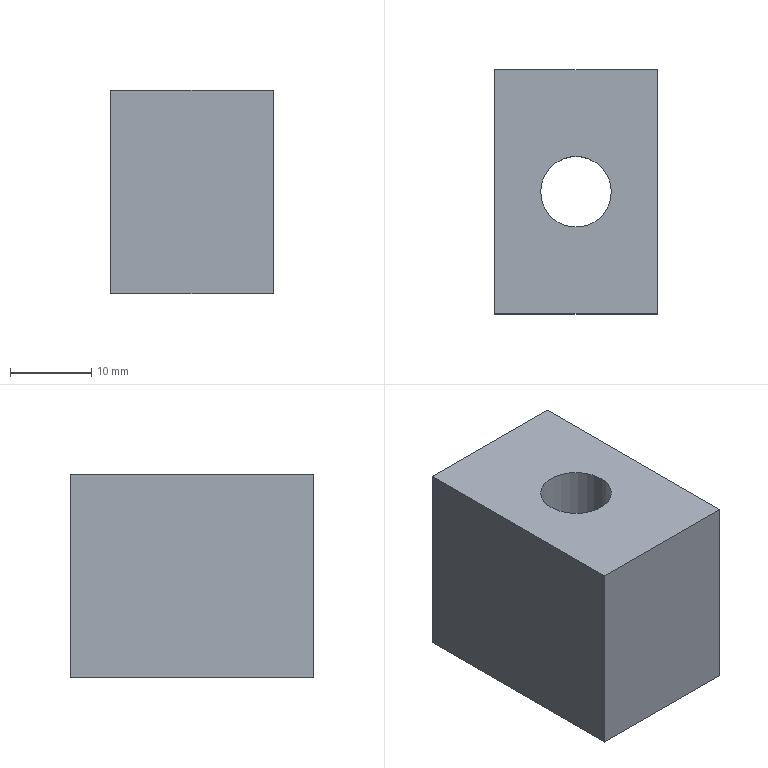Part | STEP file | 1_id1334_x_t | 1 solid | 11 faces | box 20 x 30 x 25 mm | volume 11989 mm3 | plane 7 | cylinder 4 | commonest cylinder face diameters 8.7 x2 15 x2
STEP:
#1=CARTESIAN_POINT('',(0.,0.,0.));
#2=DIRECTION('',(0.,0.,1.));
#3=DIRECTION('',(1.,0.,0.));
#4=AXIS2_PLACEMENT_3D('',#1,#2,#3);
#5=CARTESIAN_POINT('',(968.592,91.002,-86.54));
#6=VERTEX_POINT('',#5);
#7=CARTESIAN_POINT('',(948.592,91.002,-86.54));
#8=VERTEX_POINT('',#7);
#9=CARTESIAN_POINT('',(968.592,91.002,-86.54));
#10=DIRECTION('',(-1.,0.,0.));
#11=VECTOR('',#10,1.);
#12=LINE('',#9,#11);
#13=CARTESIAN_POINT('',(971.092,61.002,-86.54));
#14=DIRECTION('',(0.,0.,-1.));
#15=DIRECTION('',(1.,0.,0.));
#16=AXIS2_PLACEMENT_3D('',#13,#14,#15);
#17=PLANE('',#16);
#18=CARTESIAN_POINT('',(-2.5,-30.));
#19=DIRECTION('',(-1.,0.));
#20=VECTOR('',#19,1.);
#21=LINE('',#18,#20);
#22=(GEOMETRIC_REPRESENTATION_CONTEXT(2)PARAMETRIC_REPRESENTATION_CONTEXT()REPRESENTATION_CONTEXT('',''));
#23=DEFINITIONAL_REPRESENTATION('',(#21),#22);
#24=PCURVE('',#17,#23);
#25=CARTESIAN_POINT('',(946.092,91.002,-111.54));
#26=DIRECTION('',(0.,-1.,0.));
#27=DIRECTION('',(1.,0.,0.));
#28=AXIS2_PLACEMENT_3D('',#25,#26,#27);
#29=PLANE('',#28);
#30=CARTESIAN_POINT('',(22.5,25.));
#31=DIRECTION('',(-1.,0.));
#32=VECTOR('',#31,1.);
#33=LINE('',#30,#32);
#34=(GEOMETRIC_REPRESENTATION_CONTEXT(2)PARAMETRIC_REPRESENTATION_CONTEXT()REPRESENTATION_CONTEXT('',''));
#35=DEFINITIONAL_REPRESENTATION('',(#33),#34);
#36=PCURVE('',#29,#35);
#37=SURFACE_CURVE('',#12,(#24,#36),.PCURVE_S1.);
#38=EDGE_CURVE('',#6,#8,#37,.T.);
#39=ORIENTED_EDGE('',*,*,#38,.T.);
#40=CARTESIAN_POINT('',(948.592,61.002,-86.54));
#41=VERTEX_POINT('',#40);
#42=CARTESIAN_POINT('',(948.592,91.002,-86.54));
#43=DIRECTION('',(0.,-1.,0.));
#44=VECTOR('',#43,1.);
#45=LINE('',#42,#44);
#46=CARTESIAN_POINT('',(-22.5,-30.));
#47=DIRECTION('',(0.,1.));
#48=VECTOR('',#47,1.);
#49=LINE('',#46,#48);
#50=(GEOMETRIC_REPRESENTATION_CONTEXT(2)PARAMETRIC_REPRESENTATION_CONTEXT()REPRESENTATION_CONTEXT('',''));
#51=DEFINITIONAL_REPRESENTATION('',(#49),#50);
#52=PCURVE('',#17,#51);
#53=CARTESIAN_POINT('',(948.592,61.002,-111.54));
#54=DIRECTION('',(1.,0.,0.));
#55=DIRECTION('',(0.,0.,1.));
#56=AXIS2_PLACEMENT_3D('',#53,#54,#55);
#57=PLANE('',#56);
#58=CARTESIAN_POINT('',(25.,-30.));
#59=DIRECTION('',(0.,1.));
#60=VECTOR('',#59,1.);
#61=LINE('',#58,#60);
#62=(GEOMETRIC_REPRESENTATION_CONTEXT(2)PARAMETRIC_REPRESENTATION_CONTEXT()REPRESENTATION_CONTEXT('',''));
#63=DEFINITIONAL_REPRESENTATION('',(#61),#62);
#64=PCURVE('',#57,#63);
#65=SURFACE_CURVE('',#45,(#52,#64),.PCURVE_S1.);
#66=EDGE_CURVE('',#8,#41,#65,.T.);
#67=ORIENTED_EDGE('',*,*,#66,.T.);
#68=CARTESIAN_POINT('',(968.592,61.002,-86.54));
#69=VERTEX_POINT('',#68);
#70=CARTESIAN_POINT('',(948.592,61.002,-86.54));
#71=DIRECTION('',(1.,0.,0.));
#72=VECTOR('',#71,1.);
#73=LINE('',#70,#72);
#74=CARTESIAN_POINT('',(-22.5,0.));
#75=DIRECTION('',(1.,0.));
#76=VECTOR('',#75,1.);
#77=LINE('',#74,#76);
#78=(GEOMETRIC_REPRESENTATION_CONTEXT(2)PARAMETRIC_REPRESENTATION_CONTEXT()REPRESENTATION_CONTEXT('',''));
#79=DEFINITIONAL_REPRESENTATION('',(#77),#78);
#80=PCURVE('',#17,#79);
#81=CARTESIAN_POINT('',(971.092,61.002,-111.54));
#82=DIRECTION('',(0.,1.,0.));
#83=DIRECTION('',(0.,0.,-1.));
#84=AXIS2_PLACEMENT_3D('',#81,#82,#83);
#85=PLANE('',#84);
#86=CARTESIAN_POINT('',(-25.,22.5));
#87=DIRECTION('',(0.,-1.));
#88=VECTOR('',#87,1.);
#89=LINE('',#86,#88);
#90=(GEOMETRIC_REPRESENTATION_CONTEXT(2)PARAMETRIC_REPRESENTATION_CONTEXT()REPRESENTATION_CONTEXT('',''));
#91=DEFINITIONAL_REPRESENTATION('',(#89),#90);
#92=PCURVE('',#85,#91);
#93=SURFACE_CURVE('',#73,(#80,#92),.PCURVE_S1.);
#94=EDGE_CURVE('',#41,#69,#93,.T.);
#95=ORIENTED_EDGE('',*,*,#94,.T.);
#96=CARTESIAN_POINT('',(968.592,61.002,-86.54));
#97=DIRECTION('',(0.,1.,0.));
#98=VECTOR('',#97,1.);
#99=LINE('',#96,#98);
#100=CARTESIAN_POINT('',(-2.5,0.));
#101=DIRECTION('',(0.,-1.));
#102=VECTOR('',#101,1.);
#103=LINE('',#100,#102);
#104=(GEOMETRIC_REPRESENTATION_CONTEXT(2)PARAMETRIC_REPRESENTATION_CONTEXT()REPRESENTATION_CONTEXT('',''));
#105=DEFINITIONAL_REPRESENTATION('',(#103),#104);
#106=PCURVE('',#17,#105);
#107=CARTESIAN_POINT('',(968.592,91.002,-111.54));
#108=DIRECTION('',(-1.,0.,0.));
#109=DIRECTION('',(0.,1.,0.));
#110=AXIS2_PLACEMENT_3D('',#107,#108,#109);
#111=PLANE('',#110);
#112=CARTESIAN_POINT('',(-30.,-25.));
#113=DIRECTION('',(1.,0.));
#114=VECTOR('',#113,1.);
#115=LINE('',#112,#114);
#116=(GEOMETRIC_REPRESENTATION_CONTEXT(2)PARAMETRIC_REPRESENTATION_CONTEXT()REPRESENTATION_CONTEXT('',''));
#117=DEFINITIONAL_REPRESENTATION('',(#115),#116);
#118=PCURVE('',#111,#117);
#119=SURFACE_CURVE('',#99,(#106,#118),.PCURVE_S1.);
#120=EDGE_CURVE('',#69,#6,#119,.T.);
#121=ORIENTED_EDGE('',*,*,#120,.T.);
#122=EDGE_LOOP('',(#39,#67,#95,#121));
#123=FACE_BOUND('',#122,.T.);
#124=CARTESIAN_POINT('',(962.942,76.002,-86.54));
#125=VERTEX_POINT('',#124);
#126=CARTESIAN_POINT('',(954.242,76.002,-86.54));
#127=VERTEX_POINT('',#126);
#128=CARTESIAN_POINT('',(958.592,76.002,-86.54));
#129=DIRECTION('',(0.,0.,-1.));
#130=DIRECTION('',(1.,0.,0.));
#131=AXIS2_PLACEMENT_3D('',#128,#129,#130);
#132=CIRCLE('',#131,4.35);
#133=CARTESIAN_POINT('',(-12.5,-15.));
#134=DIRECTION('',(1.,0.));
#135=AXIS2_PLACEMENT_2D('',#133,#134);
#136=CIRCLE('',#135,4.35);
#137=(GEOMETRIC_REPRESENTATION_CONTEXT(2)PARAMETRIC_REPRESENTATION_CONTEXT()REPRESENTATION_CONTEXT('',''));
#138=DEFINITIONAL_REPRESENTATION('',(#136),#137);
#139=PCURVE('',#17,#138);
#140=CARTESIAN_POINT('',(958.592,76.002,-86.29));
#141=DIRECTION('',(0.,0.,1.));
#142=DIRECTION('',(1.,0.,0.));
#143=AXIS2_PLACEMENT_3D('',#140,#141,#142);
#144=CYLINDRICAL_SURFACE('',#143,4.35);
#145=CARTESIAN_POINT('',(6.283,-0.25));
#146=DIRECTION('',(-1.,0.));
#147=VECTOR('',#146,1.);
#148=LINE('',#145,#147);
#149=(GEOMETRIC_REPRESENTATION_CONTEXT(2)PARAMETRIC_REPRESENTATION_CONTEXT()REPRESENTATION_CONTEXT('',''));
#150=DEFINITIONAL_REPRESENTATION('',(#148),#149);
#151=PCURVE('',#144,#150);
#152=SURFACE_CURVE('',#132,(#139,#151),.PCURVE_S1.);
#153=EDGE_CURVE('',#125,#127,#152,.T.);
#154=ORIENTED_EDGE('',*,*,#153,.T.);
#155=CARTESIAN_POINT('',(958.592,76.002,-86.54));
#156=DIRECTION('',(0.,0.,-1.));
#157=DIRECTION('',(-1.,0.,0.));
#158=AXIS2_PLACEMENT_3D('',#155,#156,#157);
#159=CIRCLE('',#158,4.35);
#160=CARTESIAN_POINT('',(-12.5,-15.));
#161=DIRECTION('',(-1.,0.));
#162=AXIS2_PLACEMENT_2D('',#160,#161);
#163=CIRCLE('',#162,4.35);
#164=(GEOMETRIC_REPRESENTATION_CONTEXT(2)PARAMETRIC_REPRESENTATION_CONTEXT()REPRESENTATION_CONTEXT('',''));
#165=DEFINITIONAL_REPRESENTATION('',(#163),#164);
#166=PCURVE('',#17,#165);
#167=CARTESIAN_POINT('',(958.592,76.002,-86.29));
#168=DIRECTION('',(0.,0.,1.));
#169=DIRECTION('',(1.,0.,0.));
#170=AXIS2_PLACEMENT_3D('',#167,#168,#169);
#171=CYLINDRICAL_SURFACE('',#170,4.35);
#172=CARTESIAN_POINT('',(3.142,-0.25));
#173=DIRECTION('',(-1.,0.));
#174=VECTOR('',#173,1.);
#175=LINE('',#172,#174);
#176=(GEOMETRIC_REPRESENTATION_CONTEXT(2)PARAMETRIC_REPRESENTATION_CONTEXT()REPRESENTATION_CONTEXT('',''));
#177=DEFINITIONAL_REPRESENTATION('',(#175),#176);
#178=PCURVE('',#171,#177);
#179=SURFACE_CURVE('',#159,(#166,#178),.PCURVE_S1.);
#180=EDGE_CURVE('',#127,#125,#179,.T.);
#181=ORIENTED_EDGE('',*,*,#180,.T.);
#182=EDGE_LOOP('',(#154,#181));
#183=FACE_BOUND('',#182,.T.);
#184=ADVANCED_FACE('',(#123,#183),#17,.F.);
#185=CARTESIAN_POINT('',(968.592,61.002,-111.54));
#186=VERTEX_POINT('',#185);
#187=CARTESIAN_POINT('',(968.592,61.002,-86.54));
#188=DIRECTION('',(0.,0.,-1.));
#189=VECTOR('',#188,1.);
#190=LINE('',#187,#189);
#191=CARTESIAN_POINT('',(-30.,-25.));
#192=DIRECTION('',(0.,1.));
#193=VECTOR('',#192,1.);
#194=LINE('',#191,#193);
#195=(GEOMETRIC_REPRESENTATION_CONTEXT(2)PARAMETRIC_REPRESENTATION_CONTEXT()REPRESENTATION_CONTEXT('',''));
#196=DEFINITIONAL_REPRESENTATION('',(#194),#195);
#197=PCURVE('',#111,#196);
#198=CARTESIAN_POINT('',(-25.,2.5));
#199=DIRECTION('',(1.,0.));
#200=VECTOR('',#199,1.);
#201=LINE('',#198,#200);
#202=(GEOMETRIC_REPRESENTATION_CONTEXT(2)PARAMETRIC_REPRESENTATION_CONTEXT()REPRESENTATION_CONTEXT('',''));
#203=DEFINITIONAL_REPRESENTATION('',(#201),#202);
#204=PCURVE('',#85,#203);
#205=SURFACE_CURVE('',#190,(#197,#204),.PCURVE_S1.);
#206=EDGE_CURVE('',#69,#186,#205,.T.);
#207=ORIENTED_EDGE('',*,*,#206,.T.);
#208=CARTESIAN_POINT('',(968.592,91.002,-111.54));
#209=VERTEX_POINT('',#208);
#210=CARTESIAN_POINT('',(968.592,61.002,-111.54));
#211=DIRECTION('',(0.,1.,0.));
#212=VECTOR('',#211,1.);
#213=LINE('',#210,#212);
#214=CARTESIAN_POINT('',(-30.,0.));
#215=DIRECTION('',(1.,0.));
#216=VECTOR('',#215,1.);
#217=LINE('',#214,#216);
#218=(GEOMETRIC_REPRESENTATION_CONTEXT(2)PARAMETRIC_REPRESENTATION_CONTEXT()REPRESENTATION_CONTEXT('',''));
#219=DEFINITIONAL_REPRESENTATION('',(#217),#218);
#220=PCURVE('',#111,#219);
#221=CARTESIAN_POINT('',(971.092,61.002,-111.54));
#222=DIRECTION('',(0.,0.,-1.));
#223=DIRECTION('',(1.,0.,0.));
#224=AXIS2_PLACEMENT_3D('',#221,#222,#223);
#225=PLANE('',#224);
#226=CARTESIAN_POINT('',(-2.5,0.));
#227=DIRECTION('',(0.,-1.));
#228=VECTOR('',#227,1.);
#229=LINE('',#226,#228);
#230=(GEOMETRIC_REPRESENTATION_CONTEXT(2)PARAMETRIC_REPRESENTATION_CONTEXT()REPRESENTATION_CONTEXT('',''));
#231=DEFINITIONAL_REPRESENTATION('',(#229),#230);
#232=PCURVE('',#225,#231);
#233=SURFACE_CURVE('',#213,(#220,#232),.PCURVE_S1.);
#234=EDGE_CURVE('',#186,#209,#233,.T.);
#235=ORIENTED_EDGE('',*,*,#234,.T.);
#236=CARTESIAN_POINT('',(968.592,91.002,-86.54));
#237=DIRECTION('',(0.,0.,-1.));
#238=VECTOR('',#237,1.);
#239=LINE('',#236,#238);
#240=CARTESIAN_POINT('',(0.,-25.));
#241=DIRECTION('',(0.,1.));
#242=VECTOR('',#241,1.);
#243=LINE('',#240,#242);
#244=(GEOMETRIC_REPRESENTATION_CONTEXT(2)PARAMETRIC_REPRESENTATION_CONTEXT()REPRESENTATION_CONTEXT('',''));
#245=DEFINITIONAL_REPRESENTATION('',(#243),#244);
#246=PCURVE('',#111,#245);
#247=CARTESIAN_POINT('',(22.5,25.));
#248=DIRECTION('',(0.,-1.));
#249=VECTOR('',#248,1.);
#250=LINE('',#247,#249);
#251=(GEOMETRIC_REPRESENTATION_CONTEXT(2)PARAMETRIC_REPRESENTATION_CONTEXT()REPRESENTATION_CONTEXT('',''));
#252=DEFINITIONAL_REPRESENTATION('',(#250),#251);
#253=PCURVE('',#29,#252);
#254=SURFACE_CURVE('',#239,(#246,#253),.PCURVE_S1.);
#255=EDGE_CURVE('',#6,#209,#254,.T.);
#256=ORIENTED_EDGE('',*,*,#255,.F.);
#257=ORIENTED_EDGE('',*,*,#120,.F.);
#258=EDGE_LOOP('',(#207,#235,#256,#257));
#259=FACE_BOUND('',#258,.T.);
#260=ADVANCED_FACE('',(#259),#111,.F.);
#261=ORIENTED_EDGE('',*,*,#255,.T.);
#262=CARTESIAN_POINT('',(948.592,91.002,-111.54));
#263=VERTEX_POINT('',#262);
#264=CARTESIAN_POINT('',(968.592,91.002,-111.54));
#265=DIRECTION('',(-1.,0.,0.));
#266=VECTOR('',#265,1.);
#267=LINE('',#264,#266);
#268=CARTESIAN_POINT('',(22.5,0.));
#269=DIRECTION('',(-1.,0.));
#270=VECTOR('',#269,1.);
#271=LINE('',#268,#270);
#272=(GEOMETRIC_REPRESENTATION_CONTEXT(2)PARAMETRIC_REPRESENTATION_CONTEXT()REPRESENTATION_CONTEXT('',''));
#273=DEFINITIONAL_REPRESENTATION('',(#271),#272);
#274=PCURVE('',#29,#273);
#275=CARTESIAN_POINT('',(-2.5,-30.));
#276=DIRECTION('',(-1.,0.));
#277=VECTOR('',#276,1.);
#278=LINE('',#275,#277);
#279=(GEOMETRIC_REPRESENTATION_CONTEXT(2)PARAMETRIC_REPRESENTATION_CONTEXT()REPRESENTATION_CONTEXT('',''));
#280=DEFINITIONAL_REPRESENTATION('',(#278),#279);
#281=PCURVE('',#225,#280);
#282=SURFACE_CURVE('',#267,(#274,#281),.PCURVE_S1.);
#283=EDGE_CURVE('',#209,#263,#282,.T.);
#284=ORIENTED_EDGE('',*,*,#283,.T.);
#285=CARTESIAN_POINT('',(948.592,91.002,-86.54));
#286=DIRECTION('',(0.,0.,-1.));
#287=VECTOR('',#286,1.);
#288=LINE('',#285,#287);
#289=CARTESIAN_POINT('',(2.5,25.));
#290=DIRECTION('',(0.,-1.));
#291=VECTOR('',#290,1.);
#292=LINE('',#289,#291);
#293=(GEOMETRIC_REPRESENTATION_CONTEXT(2)PARAMETRIC_REPRESENTATION_CONTEXT()REPRESENTATION_CONTEXT('',''));
#294=DEFINITIONAL_REPRESENTATION('',(#292),#293);
#295=PCURVE('',#29,#294);
#296=CARTESIAN_POINT('',(25.,-30.));
#297=DIRECTION('',(-1.,0.));
#298=VECTOR('',#297,1.);
#299=LINE('',#296,#298);
#300=(GEOMETRIC_REPRESENTATION_CONTEXT(2)PARAMETRIC_REPRESENTATION_CONTEXT()REPRESENTATION_CONTEXT('',''));
#301=DEFINITIONAL_REPRESENTATION('',(#299),#300);
#302=PCURVE('',#57,#301);
#303=SURFACE_CURVE('',#288,(#295,#302),.PCURVE_S1.);
#304=EDGE_CURVE('',#8,#263,#303,.T.);
#305=ORIENTED_EDGE('',*,*,#304,.F.);
#306=ORIENTED_EDGE('',*,*,#38,.F.);
#307=EDGE_LOOP('',(#261,#284,#305,#306));
#308=FACE_BOUND('',#307,.T.);
#309=ADVANCED_FACE('',(#308),#29,.F.);
#310=ORIENTED_EDGE('',*,*,#304,.T.);
#311=CARTESIAN_POINT('',(948.592,61.002,-111.54));
#312=VERTEX_POINT('',#311);
#313=CARTESIAN_POINT('',(948.592,91.002,-111.54));
#314=DIRECTION('',(0.,-1.,0.));
#315=VECTOR('',#314,1.);
#316=LINE('',#313,#315);
#317=CARTESIAN_POINT('',(0.,-30.));
#318=DIRECTION('',(0.,1.));
#319=VECTOR('',#318,1.);
#320=LINE('',#317,#319);
#321=(GEOMETRIC_REPRESENTATION_CONTEXT(2)PARAMETRIC_REPRESENTATION_CONTEXT()REPRESENTATION_CONTEXT('',''));
#322=DEFINITIONAL_REPRESENTATION('',(#320),#321);
#323=PCURVE('',#57,#322);
#324=CARTESIAN_POINT('',(-22.5,-30.));
#325=DIRECTION('',(0.,1.));
#326=VECTOR('',#325,1.);
#327=LINE('',#324,#326);
#328=(GEOMETRIC_REPRESENTATION_CONTEXT(2)PARAMETRIC_REPRESENTATION_CONTEXT()REPRESENTATION_CONTEXT('',''));
#329=DEFINITIONAL_REPRESENTATION('',(#327),#328);
#330=PCURVE('',#225,#329);
#331=SURFACE_CURVE('',#316,(#323,#330),.PCURVE_S1.);
#332=EDGE_CURVE('',#263,#312,#331,.T.);
#333=ORIENTED_EDGE('',*,*,#332,.T.);
#334=CARTESIAN_POINT('',(948.592,61.002,-86.54));
#335=DIRECTION('',(0.,0.,-1.));
#336=VECTOR('',#335,1.);
#337=LINE('',#334,#336);
#338=CARTESIAN_POINT('',(25.,0.));
#339=DIRECTION('',(-1.,0.));
#340=VECTOR('',#339,1.);
#341=LINE('',#338,#340);
#342=(GEOMETRIC_REPRESENTATION_CONTEXT(2)PARAMETRIC_REPRESENTATION_CONTEXT()REPRESENTATION_CONTEXT('',''));
#343=DEFINITIONAL_REPRESENTATION('',(#341),#342);
#344=PCURVE('',#57,#343);
#345=CARTESIAN_POINT('',(-25.,22.5));
#346=DIRECTION('',(1.,0.));
#347=VECTOR('',#346,1.);
#348=LINE('',#345,#347);
#349=(GEOMETRIC_REPRESENTATION_CONTEXT(2)PARAMETRIC_REPRESENTATION_CONTEXT()REPRESENTATION_CONTEXT('',''));
#350=DEFINITIONAL_REPRESENTATION('',(#348),#349);
#351=PCURVE('',#85,#350);
#352=SURFACE_CURVE('',#337,(#344,#351),.PCURVE_S1.);
#353=EDGE_CURVE('',#41,#312,#352,.T.);
#354=ORIENTED_EDGE('',*,*,#353,.F.);
#355=ORIENTED_EDGE('',*,*,#66,.F.);
#356=EDGE_LOOP('',(#310,#333,#354,#355));
#357=FACE_BOUND('',#356,.T.);
#358=ADVANCED_FACE('',(#357),#57,.F.);
#359=ORIENTED_EDGE('',*,*,#353,.T.);
#360=CARTESIAN_POINT('',(948.592,61.002,-111.54));
#361=DIRECTION('',(1.,0.,0.));
#362=VECTOR('',#361,1.);
#363=LINE('',#360,#362);
#364=CARTESIAN_POINT('',(0.,22.5));
#365=DIRECTION('',(0.,-1.));
#366=VECTOR('',#365,1.);
#367=LINE('',#364,#366);
#368=(GEOMETRIC_REPRESENTATION_CONTEXT(2)PARAMETRIC_REPRESENTATION_CONTEXT()REPRESENTATION_CONTEXT('',''));
#369=DEFINITIONAL_REPRESENTATION('',(#367),#368);
#370=PCURVE('',#85,#369);
#371=CARTESIAN_POINT('',(-22.5,0.));
#372=DIRECTION('',(1.,0.));
#373=VECTOR('',#372,1.);
#374=LINE('',#371,#373);
#375=(GEOMETRIC_REPRESENTATION_CONTEXT(2)PARAMETRIC_REPRESENTATION_CONTEXT()REPRESENTATION_CONTEXT('',''));
#376=DEFINITIONAL_REPRESENTATION('',(#374),#375);
#377=PCURVE('',#225,#376);
#378=SURFACE_CURVE('',#363,(#370,#377),.PCURVE_S1.);
#379=EDGE_CURVE('',#312,#186,#378,.T.);
#380=ORIENTED_EDGE('',*,*,#379,.T.);
#381=ORIENTED_EDGE('',*,*,#206,.F.);
#382=ORIENTED_EDGE('',*,*,#94,.F.);
#383=EDGE_LOOP('',(#359,#380,#381,#382));
#384=FACE_BOUND('',#383,.T.);
#385=ADVANCED_FACE('',(#384),#85,.F.);
#386=ORIENTED_EDGE('',*,*,#379,.F.);
#387=ORIENTED_EDGE('',*,*,#332,.F.);
#388=ORIENTED_EDGE('',*,*,#283,.F.);
#389=ORIENTED_EDGE('',*,*,#234,.F.);
#390=EDGE_LOOP('',(#386,#387,#388,#389));
#391=FACE_BOUND('',#390,.T.);
#392=CARTESIAN_POINT('',(966.092,76.002,-111.54));
#393=VERTEX_POINT('',#392);
#394=CARTESIAN_POINT('',(951.092,76.002,-111.54));
#395=VERTEX_POINT('',#394);
#396=CARTESIAN_POINT('',(958.592,76.002,-111.54));
#397=DIRECTION('',(0.,0.,1.));
#398=DIRECTION('',(1.,0.,0.));
#399=AXIS2_PLACEMENT_3D('',#396,#397,#398);
#400=CIRCLE('',#399,7.5);
#401=CARTESIAN_POINT('',(-5.,-15.));
#402=CARTESIAN_POINT('',(-5.,-27.99));
#403=CARTESIAN_POINT('',(-16.25,-21.495));
#404=CARTESIAN_POINT('',(-27.5,-15.));
#405=CARTESIAN_POINT('',(-16.25,-8.505));
#406=CARTESIAN_POINT('',(-5.,-2.01));
#407=CARTESIAN_POINT('',(-5.,-15.));
#408=(BOUNDED_CURVE()B_SPLINE_CURVE(2,(#401,#402,#403,#404,#405,#406,#407),.UNSPECIFIED.,.T.,.F.)B_SPLINE_CURVE_WITH_KNOTS((1,2,2,2,2,1),(-2.094,0.,2.094,4.189,6.283,8.378),.UNSPECIFIED.)CURVE()GEOMETRIC_REPRESENTATION_ITEM()RATIONAL_B_SPLINE_CURVE((1.,0.5,1.,0.5,1.,0.5,1.))REPRESENTATION_ITEM(''));
#409=(GEOMETRIC_REPRESENTATION_CONTEXT(2)PARAMETRIC_REPRESENTATION_CONTEXT()REPRESENTATION_CONTEXT('',''));
#410=DEFINITIONAL_REPRESENTATION('',(#408),#409);
#411=PCURVE('',#225,#410);
#412=CARTESIAN_POINT('',(958.592,76.002,-98.54));
#413=DIRECTION('',(0.,0.,1.));
#414=DIRECTION('',(1.,0.,0.));
#415=AXIS2_PLACEMENT_3D('',#412,#413,#414);
#416=CYLINDRICAL_SURFACE('',#415,7.5);
#417=CARTESIAN_POINT('',(0.,-13.));
#418=DIRECTION('',(1.,0.));
#419=VECTOR('',#418,1.);
#420=LINE('',#417,#419);
#421=(GEOMETRIC_REPRESENTATION_CONTEXT(2)PARAMETRIC_REPRESENTATION_CONTEXT()REPRESENTATION_CONTEXT('',''));
#422=DEFINITIONAL_REPRESENTATION('',(#420),#421);
#423=PCURVE('',#416,#422);
#424=SURFACE_CURVE('',#400,(#411,#423),.PCURVE_S1.);
#425=EDGE_CURVE('',#393,#395,#424,.T.);
#426=ORIENTED_EDGE('',*,*,#425,.T.);
#427=CARTESIAN_POINT('',(958.592,76.002,-111.54));
#428=DIRECTION('',(0.,0.,1.));
#429=DIRECTION('',(-1.,0.,0.));
#430=AXIS2_PLACEMENT_3D('',#427,#428,#429);
#431=CIRCLE('',#430,7.5);
#432=CARTESIAN_POINT('',(-20.,-15.));
#433=CARTESIAN_POINT('',(-20.,-2.01));
#434=CARTESIAN_POINT('',(-8.75,-8.505));
#435=CARTESIAN_POINT('',(2.5,-15.));
#436=CARTESIAN_POINT('',(-8.75,-21.495));
#437=CARTESIAN_POINT('',(-20.,-27.99));
#438=CARTESIAN_POINT('',(-20.,-15.));
#439=(BOUNDED_CURVE()B_SPLINE_CURVE(2,(#432,#433,#434,#435,#436,#437,#438),.UNSPECIFIED.,.T.,.F.)B_SPLINE_CURVE_WITH_KNOTS((1,2,2,2,2,1),(-2.094,0.,2.094,4.189,6.283,8.378),.UNSPECIFIED.)CURVE()GEOMETRIC_REPRESENTATION_ITEM()RATIONAL_B_SPLINE_CURVE((1.,0.5,1.,0.5,1.,0.5,1.))REPRESENTATION_ITEM(''));
#440=(GEOMETRIC_REPRESENTATION_CONTEXT(2)PARAMETRIC_REPRESENTATION_CONTEXT()REPRESENTATION_CONTEXT('',''));
#441=DEFINITIONAL_REPRESENTATION('',(#439),#440);
#442=PCURVE('',#225,#441);
#443=CARTESIAN_POINT('',(958.592,76.002,-98.54));
#444=DIRECTION('',(0.,0.,1.));
#445=DIRECTION('',(1.,0.,0.));
#446=AXIS2_PLACEMENT_3D('',#443,#444,#445);
#447=CYLINDRICAL_SURFACE('',#446,7.5);
#448=CARTESIAN_POINT('',(3.142,-13.));
#449=DIRECTION('',(1.,0.));
#450=VECTOR('',#449,1.);
#451=LINE('',#448,#450);
#452=(GEOMETRIC_REPRESENTATION_CONTEXT(2)PARAMETRIC_REPRESENTATION_CONTEXT()REPRESENTATION_CONTEXT('',''));
#453=DEFINITIONAL_REPRESENTATION('',(#451),#452);
#454=PCURVE('',#447,#453);
#455=SURFACE_CURVE('',#431,(#442,#454),.PCURVE_S1.);
#456=EDGE_CURVE('',#395,#393,#455,.T.);
#457=ORIENTED_EDGE('',*,*,#456,.T.);
#458=EDGE_LOOP('',(#426,#457));
#459=FACE_BOUND('',#458,.T.);
#460=ADVANCED_FACE('',(#391,#459),#225,.T.);
#461=CARTESIAN_POINT('',(966.092,76.002,-98.54));
#462=VERTEX_POINT('',#461);
#463=CARTESIAN_POINT('',(951.092,76.002,-98.54));
#464=VERTEX_POINT('',#463);
#465=CARTESIAN_POINT('',(958.592,76.002,-98.54));
#466=DIRECTION('',(0.,0.,-1.));
#467=DIRECTION('',(1.,0.,0.));
#468=AXIS2_PLACEMENT_3D('',#465,#466,#467);
#469=CIRCLE('',#468,7.5);
#470=CARTESIAN_POINT('',(6.283,0.));
#471=DIRECTION('',(-1.,0.));
#472=VECTOR('',#471,1.);
#473=LINE('',#470,#472);
#474=(GEOMETRIC_REPRESENTATION_CONTEXT(2)PARAMETRIC_REPRESENTATION_CONTEXT()REPRESENTATION_CONTEXT('',''));
#475=DEFINITIONAL_REPRESENTATION('',(#473),#474);
#476=PCURVE('',#447,#475);
#477=CARTESIAN_POINT('',(958.592,76.002,-98.54));
#478=DIRECTION('',(0.,0.,1.));
#479=DIRECTION('',(0.,-1.,0.));
#480=AXIS2_PLACEMENT_3D('',#477,#478,#479);
#481=PLANE('',#480);
#482=CARTESIAN_POINT('',(0.,7.5));
#483=CARTESIAN_POINT('',(12.99,7.5));
#484=CARTESIAN_POINT('',(6.495,-3.75));
#485=CARTESIAN_POINT('',(0.,-15.));
#486=CARTESIAN_POINT('',(-6.495,-3.75));
#487=CARTESIAN_POINT('',(-12.99,7.5));
#488=CARTESIAN_POINT('',(0.,7.5));
#489=(BOUNDED_CURVE()B_SPLINE_CURVE(2,(#482,#483,#484,#485,#486,#487,#488),.UNSPECIFIED.,.T.,.F.)B_SPLINE_CURVE_WITH_KNOTS((1,2,2,2,2,1),(-2.094,0.,2.094,4.189,6.283,8.378),.UNSPECIFIED.)CURVE()GEOMETRIC_REPRESENTATION_ITEM()RATIONAL_B_SPLINE_CURVE((1.,0.5,1.,0.5,1.,0.5,1.))REPRESENTATION_ITEM(''));
#490=(GEOMETRIC_REPRESENTATION_CONTEXT(2)PARAMETRIC_REPRESENTATION_CONTEXT()REPRESENTATION_CONTEXT('',''));
#491=DEFINITIONAL_REPRESENTATION('',(#489),#490);
#492=PCURVE('',#481,#491);
#493=SURFACE_CURVE('',#469,(#476,#492),.PCURVE_S1.);
#494=EDGE_CURVE('',#462,#464,#493,.T.);
#495=ORIENTED_EDGE('',*,*,#494,.T.);
#496=CARTESIAN_POINT('',(951.092,76.002,-111.54));
#497=DIRECTION('',(0.,0.,-1.));
#498=VECTOR('',#497,1.);
#499=LINE('',#496,#498);
#500=CARTESIAN_POINT('',(3.142,-13.));
#501=DIRECTION('',(0.,-1.));
#502=VECTOR('',#501,1.);
#503=LINE('',#500,#502);
#504=(GEOMETRIC_REPRESENTATION_CONTEXT(2)PARAMETRIC_REPRESENTATION_CONTEXT()REPRESENTATION_CONTEXT('',''));
#505=DEFINITIONAL_REPRESENTATION('',(#503),#504);
#506=PCURVE('',#447,#505);
#507=CARTESIAN_POINT('',(3.142,-13.));
#508=DIRECTION('',(0.,-1.));
#509=VECTOR('',#508,1.);
#510=LINE('',#507,#509);
#511=(GEOMETRIC_REPRESENTATION_CONTEXT(2)PARAMETRIC_REPRESENTATION_CONTEXT()REPRESENTATION_CONTEXT('',''));
#512=DEFINITIONAL_REPRESENTATION('',(#510),#511);
#513=PCURVE('',#416,#512);
#514=SURFACE_CURVE('',#499,(#506,#513),.PCURVE_S1.);
#515=EDGE_CURVE('',#464,#395,#514,.T.);
#516=ORIENTED_EDGE('',*,*,#515,.T.);
#517=ORIENTED_EDGE('',*,*,#456,.T.);
#518=CARTESIAN_POINT('',(966.092,76.002,-111.54));
#519=DIRECTION('',(0.,0.,1.));
#520=VECTOR('',#519,1.);
#521=LINE('',#518,#520);
#522=CARTESIAN_POINT('',(6.283,-13.));
#523=DIRECTION('',(0.,1.));
#524=VECTOR('',#523,1.);
#525=LINE('',#522,#524);
#526=(GEOMETRIC_REPRESENTATION_CONTEXT(2)PARAMETRIC_REPRESENTATION_CONTEXT()REPRESENTATION_CONTEXT('',''));
#527=DEFINITIONAL_REPRESENTATION('',(#525),#526);
#528=PCURVE('',#447,#527);
#529=CARTESIAN_POINT('',(0.,-13.));
#530=DIRECTION('',(0.,1.));
#531=VECTOR('',#530,1.);
#532=LINE('',#529,#531);
#533=(GEOMETRIC_REPRESENTATION_CONTEXT(2)PARAMETRIC_REPRESENTATION_CONTEXT()REPRESENTATION_CONTEXT('',''));
#534=DEFINITIONAL_REPRESENTATION('',(#532),#533);
#535=PCURVE('',#416,#534);
#536=SURFACE_CURVE('',#521,(#528,#535),.PCURVE_S1.);
#537=EDGE_CURVE('',#393,#462,#536,.T.);
#538=ORIENTED_EDGE('',*,*,#537,.T.);
#539=EDGE_LOOP('',(#495,#516,#517,#538));
#540=FACE_BOUND('',#539,.F.);
#541=ADVANCED_FACE('',(#540),#447,.F.);
#542=ORIENTED_EDGE('',*,*,#494,.T.);
#543=CARTESIAN_POINT('',(958.592,76.002,-98.54));
#544=DIRECTION('',(0.,0.,-1.));
#545=DIRECTION('',(-1.,0.,0.));
#546=AXIS2_PLACEMENT_3D('',#543,#544,#545);
#547=CIRCLE('',#546,7.5);
#548=CARTESIAN_POINT('',(0.,-7.5));
#549=CARTESIAN_POINT('',(-12.99,-7.5));
#550=CARTESIAN_POINT('',(-6.495,3.75));
#551=CARTESIAN_POINT('',(0.,15.));
#552=CARTESIAN_POINT('',(6.495,3.75));
#553=CARTESIAN_POINT('',(12.99,-7.5));
#554=CARTESIAN_POINT('',(0.,-7.5));
#555=(BOUNDED_CURVE()B_SPLINE_CURVE(2,(#548,#549,#550,#551,#552,#553,#554),.UNSPECIFIED.,.T.,.F.)B_SPLINE_CURVE_WITH_KNOTS((1,2,2,2,2,1),(-2.094,0.,2.094,4.189,6.283,8.378),.UNSPECIFIED.)CURVE()GEOMETRIC_REPRESENTATION_ITEM()RATIONAL_B_SPLINE_CURVE((1.,0.5,1.,0.5,1.,0.5,1.))REPRESENTATION_ITEM(''));
#556=(GEOMETRIC_REPRESENTATION_CONTEXT(2)PARAMETRIC_REPRESENTATION_CONTEXT()REPRESENTATION_CONTEXT('',''));
#557=DEFINITIONAL_REPRESENTATION('',(#555),#556);
#558=PCURVE('',#481,#557);
#559=CARTESIAN_POINT('',(3.142,0.));
#560=DIRECTION('',(-1.,0.));
#561=VECTOR('',#560,1.);
#562=LINE('',#559,#561);
#563=(GEOMETRIC_REPRESENTATION_CONTEXT(2)PARAMETRIC_REPRESENTATION_CONTEXT()REPRESENTATION_CONTEXT('',''));
#564=DEFINITIONAL_REPRESENTATION('',(#562),#563);
#565=PCURVE('',#416,#564);
#566=SURFACE_CURVE('',#547,(#558,#565),.PCURVE_S1.);
#567=EDGE_CURVE('',#464,#462,#566,.T.);
#568=ORIENTED_EDGE('',*,*,#567,.T.);
#569=EDGE_LOOP('',(#542,#568));
#570=FACE_BOUND('',#569,.T.);
#571=CARTESIAN_POINT('',(954.242,76.002,-98.54));
#572=VERTEX_POINT('',#571);
#573=CARTESIAN_POINT('',(962.942,76.002,-98.54));
#574=VERTEX_POINT('',#573);
#575=CARTESIAN_POINT('',(958.592,76.002,-98.54));
#576=DIRECTION('',(0.,0.,1.));
#577=DIRECTION('',(-1.,0.,0.));
#578=AXIS2_PLACEMENT_3D('',#575,#576,#577);
#579=CIRCLE('',#578,4.35);
#580=CARTESIAN_POINT('',(0.,0.));
#581=DIRECTION('',(0.,-1.));
#582=AXIS2_PLACEMENT_2D('',#580,#581);
#583=CIRCLE('',#582,4.35);
#584=(GEOMETRIC_REPRESENTATION_CONTEXT(2)PARAMETRIC_REPRESENTATION_CONTEXT()REPRESENTATION_CONTEXT('',''));
#585=DEFINITIONAL_REPRESENTATION('',(#583),#584);
#586=PCURVE('',#481,#585);
#587=CARTESIAN_POINT('',(3.142,-12.25));
#588=DIRECTION('',(1.,0.));
#589=VECTOR('',#588,1.);
#590=LINE('',#587,#589);
#591=(GEOMETRIC_REPRESENTATION_CONTEXT(2)PARAMETRIC_REPRESENTATION_CONTEXT()REPRESENTATION_CONTEXT('',''));
#592=DEFINITIONAL_REPRESENTATION('',(#590),#591);
#593=PCURVE('',#144,#592);
#594=SURFACE_CURVE('',#579,(#586,#593),.PCURVE_S1.);
#595=EDGE_CURVE('',#572,#574,#594,.T.);
#596=ORIENTED_EDGE('',*,*,#595,.T.);
#597=CARTESIAN_POINT('',(958.592,76.002,-98.54));
#598=DIRECTION('',(0.,0.,1.));
#599=DIRECTION('',(1.,0.,0.));
#600=AXIS2_PLACEMENT_3D('',#597,#598,#599);
#601=CIRCLE('',#600,4.35);
#602=CARTESIAN_POINT('',(0.,0.));
#603=DIRECTION('',(0.,1.));
#604=AXIS2_PLACEMENT_2D('',#602,#603);
#605=CIRCLE('',#604,4.35);
#606=(GEOMETRIC_REPRESENTATION_CONTEXT(2)PARAMETRIC_REPRESENTATION_CONTEXT()REPRESENTATION_CONTEXT('',''));
#607=DEFINITIONAL_REPRESENTATION('',(#605),#606);
#608=PCURVE('',#481,#607);
#609=CARTESIAN_POINT('',(0.,-12.25));
#610=DIRECTION('',(1.,0.));
#611=VECTOR('',#610,1.);
#612=LINE('',#609,#611);
#613=(GEOMETRIC_REPRESENTATION_CONTEXT(2)PARAMETRIC_REPRESENTATION_CONTEXT()REPRESENTATION_CONTEXT('',''));
#614=DEFINITIONAL_REPRESENTATION('',(#612),#613);
#615=PCURVE('',#171,#614);
#616=SURFACE_CURVE('',#601,(#608,#615),.PCURVE_S1.);
#617=EDGE_CURVE('',#574,#572,#616,.T.);
#618=ORIENTED_EDGE('',*,*,#617,.T.);
#619=EDGE_LOOP('',(#596,#618));
#620=FACE_BOUND('',#619,.T.);
#621=ADVANCED_FACE('',(#570,#620),#481,.F.);
#622=ORIENTED_EDGE('',*,*,#567,.T.);
#623=ORIENTED_EDGE('',*,*,#537,.F.);
#624=ORIENTED_EDGE('',*,*,#425,.T.);
#625=ORIENTED_EDGE('',*,*,#515,.F.);
#626=EDGE_LOOP('',(#622,#623,#624,#625));
#627=FACE_BOUND('',#626,.F.);
#628=ADVANCED_FACE('',(#627),#416,.F.);
#629=ORIENTED_EDGE('',*,*,#180,.T.);
#630=CARTESIAN_POINT('',(962.942,76.002,-98.54));
#631=DIRECTION('',(0.,0.,1.));
#632=VECTOR('',#631,1.);
#633=LINE('',#630,#632);
#634=CARTESIAN_POINT('',(0.,-12.25));
#635=DIRECTION('',(0.,1.));
#636=VECTOR('',#635,1.);
#637=LINE('',#634,#636);
#638=(GEOMETRIC_REPRESENTATION_CONTEXT(2)PARAMETRIC_REPRESENTATION_CONTEXT()REPRESENTATION_CONTEXT('',''));
#639=DEFINITIONAL_REPRESENTATION('',(#637),#638);
#640=PCURVE('',#171,#639);
#641=CARTESIAN_POINT('',(6.283,-12.25));
#642=DIRECTION('',(0.,1.));
#643=VECTOR('',#642,1.);
#644=LINE('',#641,#643);
#645=(GEOMETRIC_REPRESENTATION_CONTEXT(2)PARAMETRIC_REPRESENTATION_CONTEXT()REPRESENTATION_CONTEXT('',''));
#646=DEFINITIONAL_REPRESENTATION('',(#644),#645);
#647=PCURVE('',#144,#646);
#648=SURFACE_CURVE('',#633,(#640,#647),.PCURVE_S1.);
#649=EDGE_CURVE('',#574,#125,#648,.T.);
#650=ORIENTED_EDGE('',*,*,#649,.F.);
#651=ORIENTED_EDGE('',*,*,#617,.T.);
#652=CARTESIAN_POINT('',(954.242,76.002,-98.54));
#653=DIRECTION('',(0.,0.,-1.));
#654=VECTOR('',#653,1.);
#655=LINE('',#652,#654);
#656=CARTESIAN_POINT('',(3.142,-12.25));
#657=DIRECTION('',(0.,-1.));
#658=VECTOR('',#657,1.);
#659=LINE('',#656,#658);
#660=(GEOMETRIC_REPRESENTATION_CONTEXT(2)PARAMETRIC_REPRESENTATION_CONTEXT()REPRESENTATION_CONTEXT('',''));
#661=DEFINITIONAL_REPRESENTATION('',(#659),#660);
#662=PCURVE('',#171,#661);
#663=CARTESIAN_POINT('',(3.142,-12.25));
#664=DIRECTION('',(0.,-1.));
#665=VECTOR('',#664,1.);
#666=LINE('',#663,#665);
#667=(GEOMETRIC_REPRESENTATION_CONTEXT(2)PARAMETRIC_REPRESENTATION_CONTEXT()REPRESENTATION_CONTEXT('',''));
#668=DEFINITIONAL_REPRESENTATION('',(#666),#667);
#669=PCURVE('',#144,#668);
#670=SURFACE_CURVE('',#655,(#662,#669),.PCURVE_S1.);
#671=EDGE_CURVE('',#127,#572,#670,.T.);
#672=ORIENTED_EDGE('',*,*,#671,.F.);
#673=EDGE_LOOP('',(#629,#650,#651,#672));
#674=FACE_BOUND('',#673,.F.);
#675=ADVANCED_FACE('',(#674),#171,.F.);
#676=ORIENTED_EDGE('',*,*,#153,.T.);
#677=ORIENTED_EDGE('',*,*,#671,.T.);
#678=ORIENTED_EDGE('',*,*,#595,.T.);
#679=ORIENTED_EDGE('',*,*,#649,.T.);
#680=EDGE_LOOP('',(#676,#677,#678,#679));
#681=FACE_BOUND('',#680,.F.);
#682=ADVANCED_FACE('',(#681),#144,.F.);
#683=CLOSED_SHELL('',(#184,#260,#309,#358,#385,#460,#541,#621,#628,#675,#682));
#684=MANIFOLD_SOLID_BREP('',#683);
#685=(LENGTH_UNIT()NAMED_UNIT(*)SI_UNIT(.MILLI.,.METRE.));
#686=UNCERTAINTY_MEASURE_WITH_UNIT(LENGTH_MEASURE(0.0000001),#685,'','');
#687=(NAMED_UNIT(*)PLANE_ANGLE_UNIT()SI_UNIT($,.RADIAN.));
#688=(NAMED_UNIT(*)SI_UNIT($,.STERADIAN.)SOLID_ANGLE_UNIT());
#689=(GEOMETRIC_REPRESENTATION_CONTEXT(3)GLOBAL_UNCERTAINTY_ASSIGNED_CONTEXT((#686))GLOBAL_UNIT_ASSIGNED_CONTEXT((#685,#687,#688))REPRESENTATION_CONTEXT('',''));
#690=ADVANCED_BREP_SHAPE_REPRESENTATION('',(#4,#684),#689);